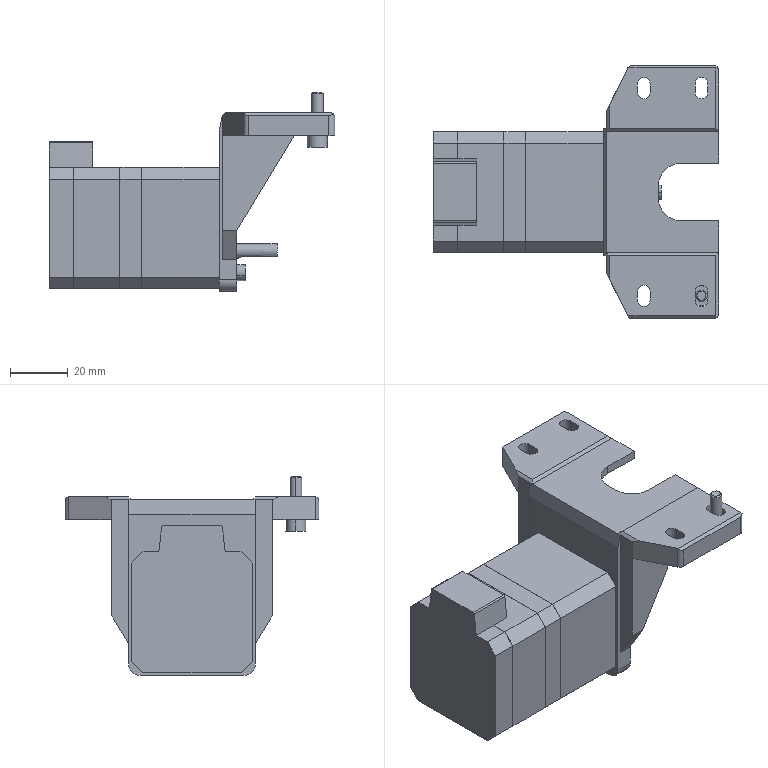Part | SolidWorks | features AEMSimFeature 1 | 4 solids | 242 faces | box 99 x 88 x 69 mm | volume 136983 mm3 | plane 162 | cylinder 64 | cone 16 | commonest cylinder face diameters 1 x14 2.5 x8 3.5 x8 4.4 x8 4 x6 8 x3